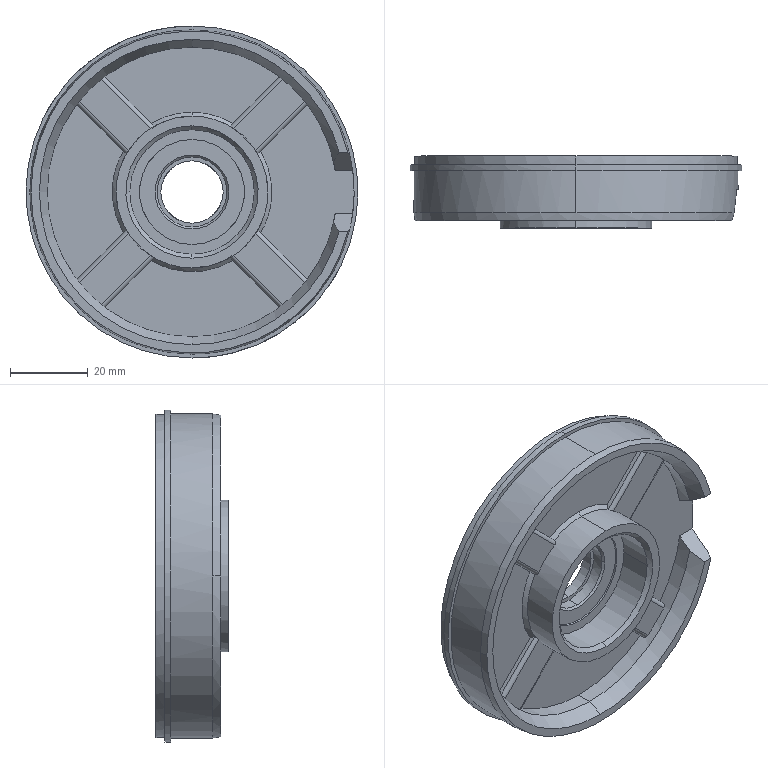Part | STEP file | 1 solid | 95 faces | box 85.3 x 18.5 x 85.3 mm | volume 37197 mm3 | cylinder 45 | plane 34 | cone 14 | spline 2 | commonest cylinder face diameters 2 x17 75 x4 71 x3 74.4 x3 16 x2 18 x2